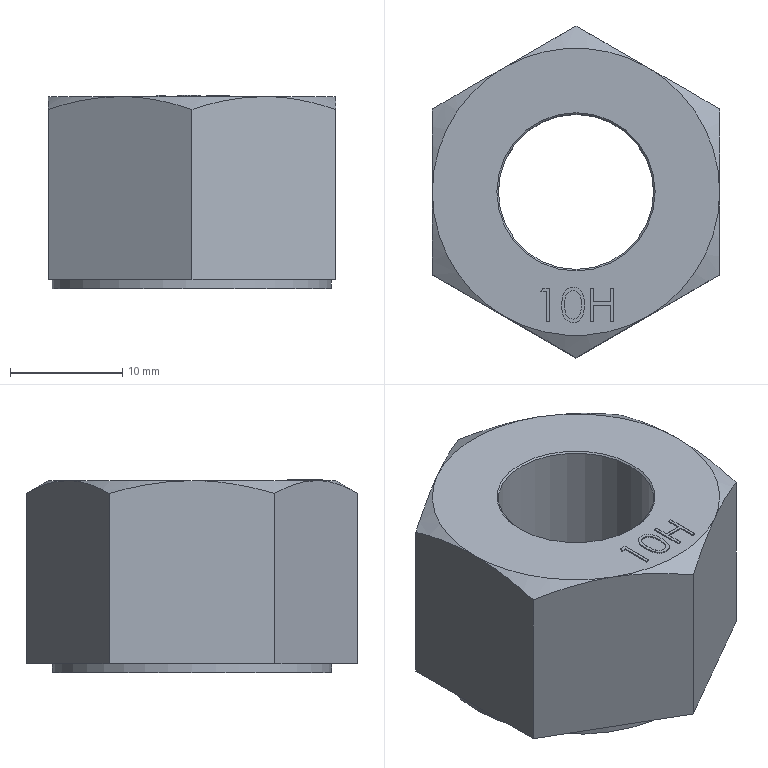Part | STEP file | Hex nut for steel structures M16 10H GBT1229-2006_M16 | 1 solid | 50 faces | box 25.6 x 29.56 x 17.2 mm | volume 7051 mm3 | plane 31 | spline 9 | cone 8 | cylinder 2 | commonest cylinder face diameters 13.835 x1 24.9 x1